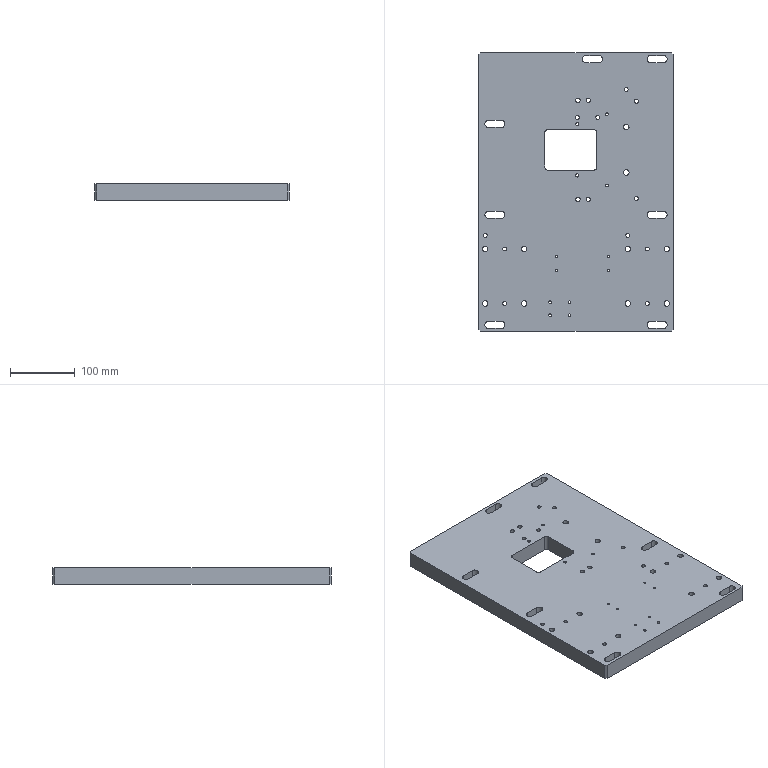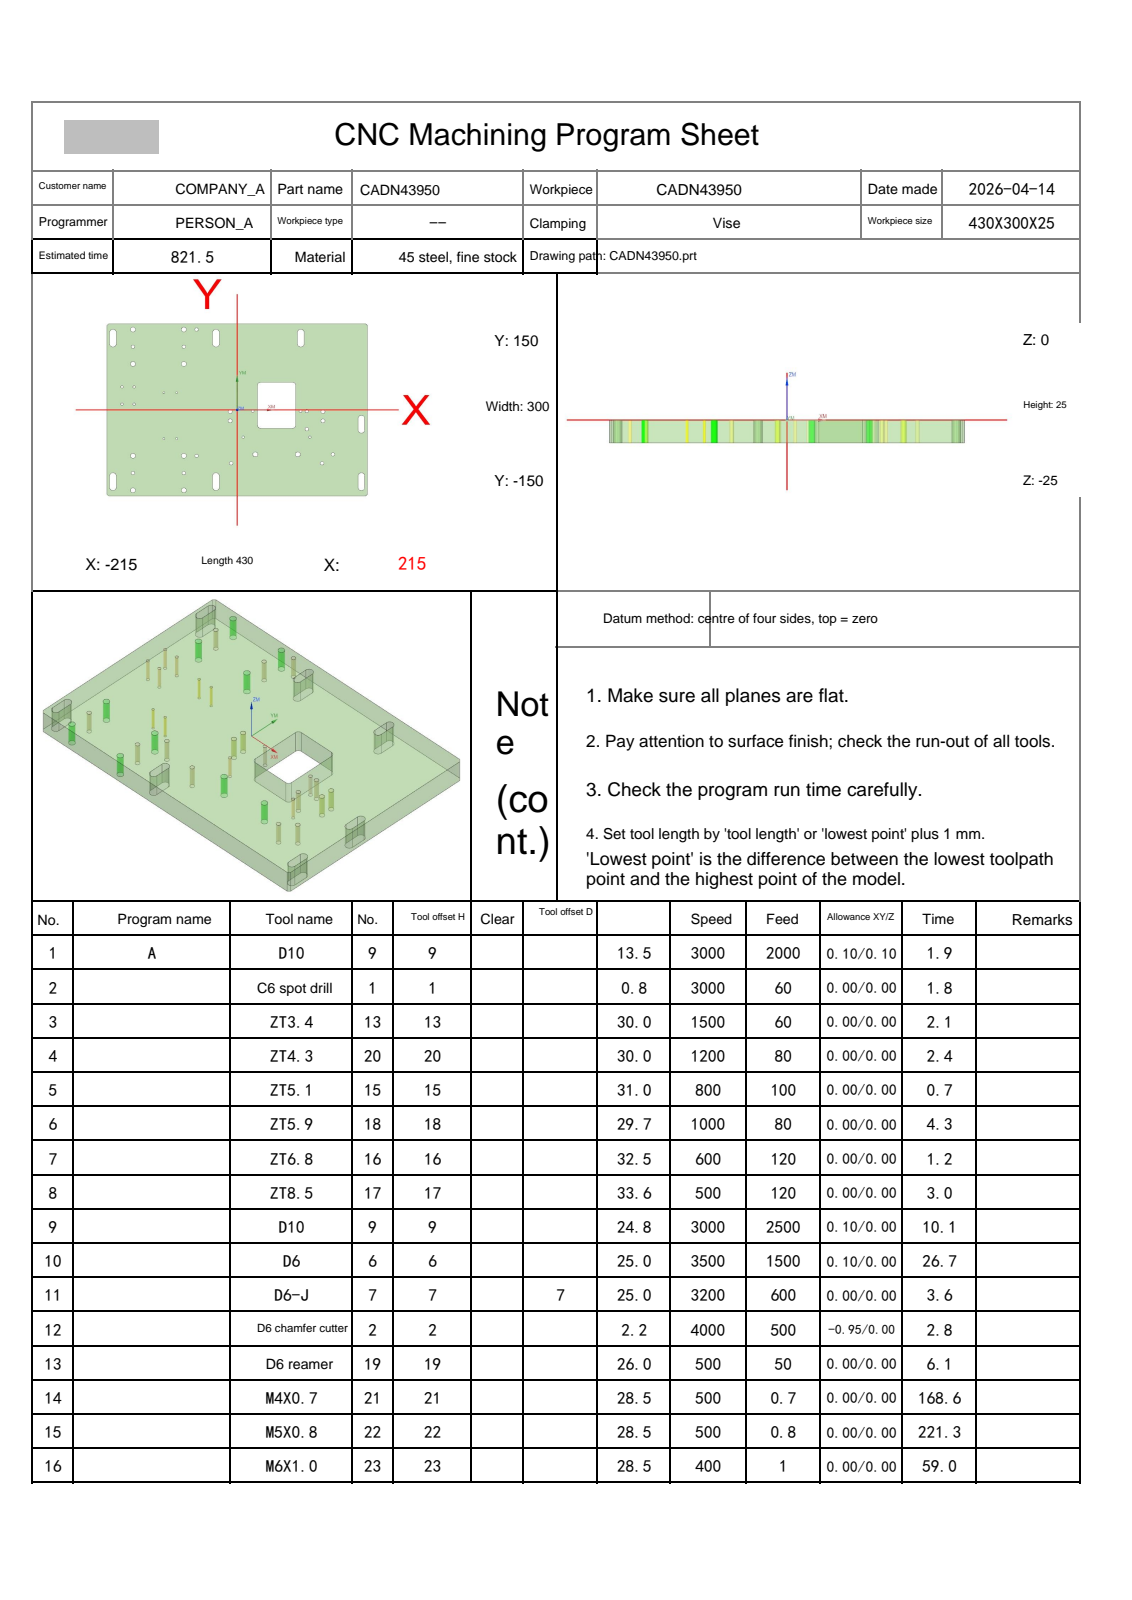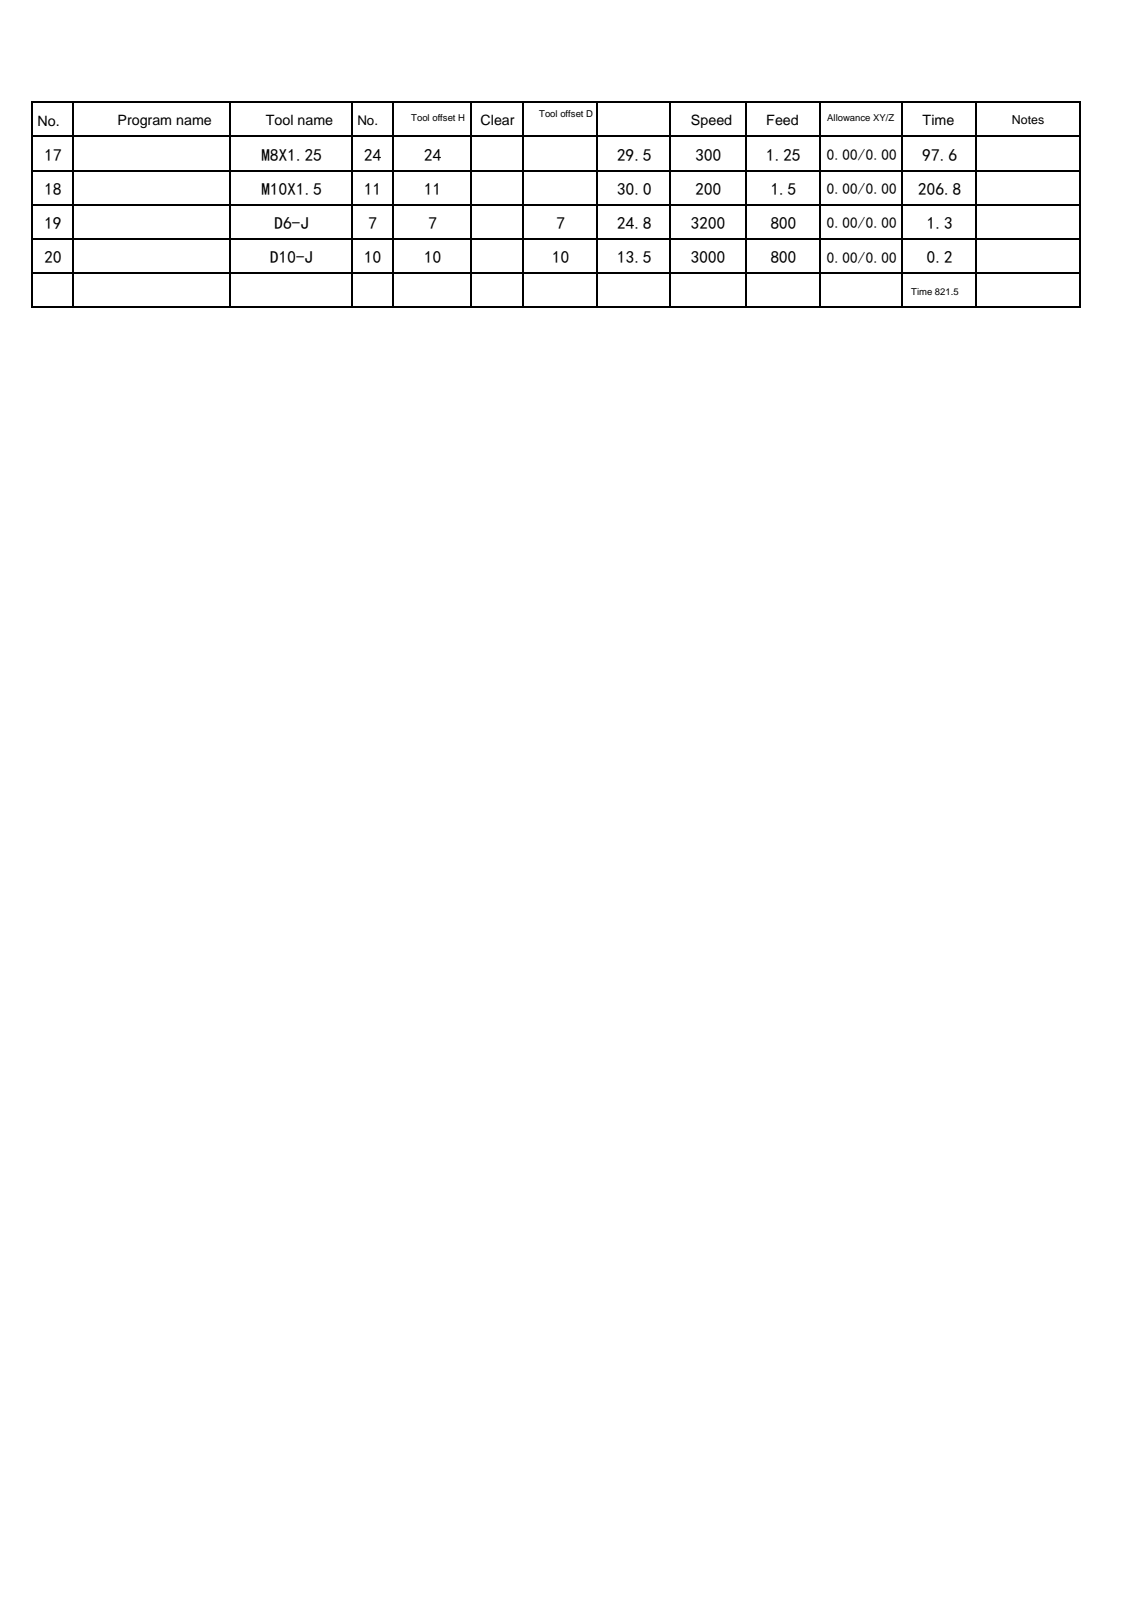NC program | NX | posted by the shop | part box 300 x 430 x 25 mm
Lines 5671 to 7024 of 7024:
N11 T07 M06
(D6-J  D=6. R=0. H=07 ce=0.00 di=0.00)
G00 G90 G54 X-207.25 Y-124.8 M03 S3200
G43 H07 Z20.
M08
Z-4.5
G01 Z-5. F600.
G41 D07
X-207.3
G03 X-207.5 Y-125. I0.0 J-.2
G01 Y-135.
G03 X-205. Y-137.5 I2.5 J0.0
X-202.5 Y-135. I0.0 J2.5
G01 Y-115.
G03 X-205. Y-112.5 I-2.5 J0.0
X-207.5 Y-115. I0.0 J-2.5
G01 Y-125.
Y-125.5
G03 X-207.3 Y-125.7 I.2 J0.0
G01 G40 X-207.25
Z-4.5
G00 Z1.
Y-124.8
Z-9.5
G01 Z-10.
G41 D07
X-207.3
G03 X-207.5 Y-125. I0.0 J-.2
G01 Y-135.
G03 X-205. Y-137.5 I2.5 J0.0
X-202.5 Y-135. I0.0 J2.5
G01 Y-115.
G03 X-205. Y-112.5 I-2.5 J0.0
X-207.5 Y-115. I0.0 J-2.5
G01 Y-125.
Y-125.5
G03 X-207.3 Y-125.7 I.2 J0.0
G01 G40 X-207.25
Z-9.5
G00 Z-4.
Y-124.8
Z-14.5
G01 Z-15.
G41 D07
X-207.3
G03 X-207.5 Y-125. I0.0 J-.2
G01 Y-135.
G03 X-205. Y-137.5 I2.5 J0.0
X-202.5 Y-135. I0.0 J2.5
G01 Y-115.
G03 X-205. Y-112.5 I-2.5 J0.0
X-207.5 Y-115. I0.0 J-2.5
G01 Y-125.
Y-125.5
G03 X-207.3 Y-125.7 I.2 J0.0
G01 G40 X-207.25
Z-14.5
G00 Z-9.
Y-124.8
Z-19.5
G01 Z-20.
G41 D07
X-207.3
G03 X-207.5 Y-125. I0.0 J-.2
G01 Y-135.
G03 X-205. Y-137.5 I2.5 J0.0
X-202.5 Y-135. I0.0 J2.5
G01 Y-115.
G03 X-205. Y-112.5 I-2.5 J0.0
X-207.5 Y-115. I0.0 J-2.5
G01 Y-125.
Y-125.5
G03 X-207.3 Y-125.7 I.2 J0.0
G01 G40 X-207.25
Z-19.5
G00 Z-14.
Y-124.8
Z-24.5
G01 Z-25.
G41 D07
X-207.3
G03 X-207.5 Y-125. I0.0 J-.2
G01 Y-135.
G03 X-205. Y-137.5 I2.5 J0.0
X-202.5 Y-135. I0.0 J2.5
G01 Y-115.
G03 X-205. Y-112.5 I-2.5 J0.0
X-207.5 Y-115. I0.0 J-2.5
G01 Y-125.
Y-125.5
G03 X-207.3 Y-125.7 I.2 J0.0
G01 G40 X-207.25
Z-24.5
G00 Z20.
X-37.25 Y-124.8
Z-4.5
G01 Z-5.
G41 D07
X-37.3
G03 X-37.5 Y-125. I0.0 J-.2
G01 Y-135.
G03 X-35. Y-137.5 I2.5 J0.0
X-32.5 Y-135. I0.0 J2.5
G01 Y-115.
G03 X-35. Y-112.5 I-2.5 J0.0
X-37.5 Y-115. I0.0 J-2.5
G01 Y-125.
Y-125.5
G03 X-37.3 Y-125.7 I.2 J0.0
G01 G40 X-37.25
Z-4.5
G00 Z1.
Y-124.8
Z-9.5
G01 Z-10.
G41 D07
X-37.3
G03 X-37.5 Y-125. I0.0 J-.2
G01 Y-135.
G03 X-35. Y-137.5 I2.5 J0.0
X-32.5 Y-135. I0.0 J2.5
G01 Y-115.
G03 X-35. Y-112.5 I-2.5 J0.0
X-37.5 Y-115. I0.0 J-2.5
G01 Y-125.
Y-125.5
G03 X-37.3 Y-125.7 I.2 J0.0
G01 G40 X-37.25
Z-9.5
G00 Z-4.
Y-124.8
Z-14.5
G01 Z-15.
G41 D07
X-37.3
G03 X-37.5 Y-125. I0.0 J-.2
G01 Y-135.
G03 X-35. Y-137.5 I2.5 J0.0
X-32.5 Y-135. I0.0 J2.5
G01 Y-115.
G03 X-35. Y-112.5 I-2.5 J0.0
X-37.5 Y-115. I0.0 J-2.5
G01 Y-125.
Y-125.5
G03 X-37.3 Y-125.7 I.2 J0.0
G01 G40 X-37.25
Z-14.5
G00 Z-9.
Y-124.8
Z-19.5
G01 Z-20.
G41 D07
X-37.3
G03 X-37.5 Y-125. I0.0 J-.2
G01 Y-135.
G03 X-35. Y-137.5 I2.5 J0.0
X-32.5 Y-135. I0.0 J2.5
G01 Y-115.
G03 X-35. Y-112.5 I-2.5 J0.0
X-37.5 Y-115. I0.0 J-2.5
G01 Y-125.
Y-125.5
G03 X-37.3 Y-125.7 I.2 J0.0
G01 G40 X-37.25
Z-19.5
G00 Z-14.
Y-124.8
Z-24.5
G01 Z-25.
G41 D07
X-37.3
G03 X-37.5 Y-125. I0.0 J-.2
G01 Y-135.
G03 X-35. Y-137.5 I2.5 J0.0
X-32.5 Y-135. I0.0 J2.5
G01 Y-115.
G03 X-35. Y-112.5 I-2.5 J0.0
X-37.5 Y-115. I0.0 J-2.5
G01 Y-125.
Y-125.5
G03 X-37.3 Y-125.7 I.2 J0.0
G01 G40 X-37.25
Z-24.5
G00 Z20.
X207.25 Y-125.2
Z-4.5
G01 Z-5.
G41 D07
X207.3
G03 X207.5 Y-125. I0.0 J.2
G01 Y-115.
G03 X205. Y-112.5 I-2.5 J0.0
X202.5 Y-115. I0.0 J-2.5
G01 Y-135.
G03 X205. Y-137.5 I2.5 J0.0
X207.5 Y-135. I0.0 J2.5
G01 Y-125.
Y-124.5
G03 X207.3 Y-124.3 I-.2 J0.0
G01 G40 X207.25
Z-4.5
G00 Z1.
Y-125.2
Z-9.5
G01 Z-10.
G41 D07
X207.3
G03 X207.5 Y-125. I0.0 J.2
G01 Y-115.
G03 X205. Y-112.5 I-2.5 J0.0
X202.5 Y-115. I0.0 J-2.5
G01 Y-135.
G03 X205. Y-137.5 I2.5 J0.0
X207.5 Y-135. I0.0 J2.5
G01 Y-125.
Y-124.5
G03 X207.3 Y-124.3 I-.2 J0.0
G01 G40 X207.25
Z-9.5
G00 Z-4.
Y-125.2
Z-14.5
G01 Z-15.
G41 D07
X207.3
G03 X207.5 Y-125. I0.0 J.2
G01 Y-115.
G03 X205. Y-112.5 I-2.5 J0.0
X202.5 Y-115. I0.0 J-2.5
G01 Y-135.
G03 X205. Y-137.5 I2.5 J0.0
X207.5 Y-135. I0.0 J2.5
G01 Y-125.
Y-124.5
G03 X207.3 Y-124.3 I-.2 J0.0
G01 G40 X207.25
Z-14.5
G00 Z-9.
Y-125.2
Z-19.5
G01 Z-20.
G41 D07
X207.3
G03 X207.5 Y-125. I0.0 J.2
G01 Y-115.
G03 X205. Y-112.5 I-2.5 J0.0
X202.5 Y-115. I0.0 J-2.5
G01 Y-135.
G03 X205. Y-137.5 I2.5 J0.0
X207.5 Y-135. I0.0 J2.5
G01 Y-125.
Y-124.5
G03 X207.3 Y-124.3 I-.2 J0.0
G01 G40 X207.25
Z-19.5
G00 Z-14.
Y-125.2
Z-24.5
G01 Z-25.
G41 D07
X207.3
G03 X207.5 Y-125. I0.0 J.2
G01 Y-115.
G03 X205. Y-112.5 I-2.5 J0.0
X202.5 Y-115. I0.0 J-2.5
G01 Y-135.
G03 X205. Y-137.5 I2.5 J0.0
X207.5 Y-135. I0.0 J2.5
G01 Y-125.
Y-124.5
G03 X207.3 Y-124.3 I-.2 J0.0
G01 G40 X207.25
Z-24.5
G00 Z20.
Y-25.2
Z-4.5
G01 Z-5.
G41 D07
X207.3
G03 X207.5 Y-25. I0.0 J.2
G01 Y-15.
G03 X205. Y-12.5 I-2.5 J0.0
X202.5 Y-15. I0.0 J-2.5
G01 Y-35.
G03 X205. Y-37.5 I2.5 J0.0
X207.5 Y-35. I0.0 J2.5
G01 Y-25.
Y-24.5
G03 X207.3 Y-24.3 I-.2 J0.0
G01 G40 X207.25
Z-4.5
G00 Z1.
Y-25.2
Z-9.5
G01 Z-10.
G41 D07
X207.3
G03 X207.5 Y-25. I0.0 J.2
G01 Y-15.
G03 X205. Y-12.5 I-2.5 J0.0
X202.5 Y-15. I0.0 J-2.5
G01 Y-35.
G03 X205. Y-37.5 I2.5 J0.0
X207.5 Y-35. I0.0 J2.5
G01 Y-25.
Y-24.5
G03 X207.3 Y-24.3 I-.2 J0.0
G01 G40 X207.25
Z-9.5
G00 Z-4.
Y-25.2
Z-14.5
G01 Z-15.
G41 D07
X207.3
G03 X207.5 Y-25. I0.0 J.2
G01 Y-15.
G03 X205. Y-12.5 I-2.5 J0.0
X202.5 Y-15. I0.0 J-2.5
G01 Y-35.
G03 X205. Y-37.5 I2.5 J0.0
X207.5 Y-35. I0.0 J2.5
G01 Y-25.
Y-24.5
G03 X207.3 Y-24.3 I-.2 J0.0
G01 G40 X207.25
Z-14.5
G00 Z-9.
Y-25.2
Z-19.5
G01 Z-20.
G41 D07
X207.3
G03 X207.5 Y-25. I0.0 J.2
G01 Y-15.
G03 X205. Y-12.5 I-2.5 J0.0
X202.5 Y-15. I0.0 J-2.5
G01 Y-35.
G03 X205. Y-37.5 I2.5 J0.0
X207.5 Y-35. I0.0 J2.5
G01 Y-25.
Y-24.5
G03 X207.3 Y-24.3 I-.2 J0.0
G01 G40 X207.25
Z-19.5
G00 Z-14.
Y-25.2
Z-24.5
G01 Z-25.
G41 D07
X207.3
G03 X207.5 Y-25. I0.0 J.2
G01 Y-15.
G03 X205. Y-12.5 I-2.5 J0.0
X202.5 Y-15. I0.0 J-2.5
G01 Y-35.
G03 X205. Y-37.5 I2.5 J0.0
X207.5 Y-35. I0.0 J2.5
G01 Y-25.
Y-24.5
G03 X207.3 Y-24.3 I-.2 J0.0
G01 G40 X207.25
Z-24.5
G00 Z20.
X107.25 Y124.8
Z-4.5
G01 Z-5.
G41 D07
X107.3
G03 X107.5 Y125. I0.0 J.2
G01 Y135.
G03 X105. Y137.5 I-2.5 J0.0
X102.5 Y135. I0.0 J-2.5
G01 Y115.
G03 X105. Y112.5 I2.5 J0.0
X107.5 Y115. I0.0 J2.5
G01 Y125.
Y125.5
G03 X107.3 Y125.7 I-.2 J0.0
G01 G40 X107.25
Z-4.5
G00 Z1.
Y124.8
Z-9.5
G01 Z-10.
G41 D07
X107.3
G03 X107.5 Y125. I0.0 J.2
G01 Y135.
G03 X105. Y137.5 I-2.5 J0.0
X102.5 Y135. I0.0 J-2.5
G01 Y115.
G03 X105. Y112.5 I2.5 J0.0
X107.5 Y115. I0.0 J2.5
G01 Y125.
Y125.5
G03 X107.3 Y125.7 I-.2 J0.0
G01 G40 X107.25
Z-9.5
G00 Z-4.
Y124.8
Z-14.5
G01 Z-15.
G41 D07
X107.3
G03 X107.5 Y125. I0.0 J.2
G01 Y135.
G03 X105. Y137.5 I-2.5 J0.0
X102.5 Y135. I0.0 J-2.5
G01 Y115.
G03 X105. Y112.5 I2.5 J0.0
X107.5 Y115. I0.0 J2.5
G01 Y125.
Y125.5
G03 X107.3 Y125.7 I-.2 J0.0
G01 G40 X107.25
Z-14.5
G00 Z-9.
Y124.8
Z-19.5
G01 Z-20.
G41 D07
X107.3
G03 X107.5 Y125. I0.0 J.2
G01 Y135.
G03 X105. Y137.5 I-2.5 J0.0
X102.5 Y135. I0.0 J-2.5
G01 Y115.
G03 X105. Y112.5 I2.5 J0.0
X107.5 Y115. I0.0 J2.5
G01 Y125.
Y125.5
G03 X107.3 Y125.7 I-.2 J0.0
G01 G40 X107.25
Z-19.5
G00 Z-14.
Y124.8
Z-24.5
G01 Z-25.
G41 D07
X107.3
G03 X107.5 Y125. I0.0 J.2
G01 Y135.
G03 X105. Y137.5 I-2.5 J0.0
X102.5 Y135. I0.0 J-2.5
G01 Y115.
G03 X105. Y112.5 I2.5 J0.0
X107.5 Y115. I0.0 J2.5
G01 Y125.
Y125.5
G03 X107.3 Y125.7 I-.2 J0.0
G01 G40 X107.25
Z-24.5
G00 Z20.
X-32.75 Y124.8
Z-4.5
G01 Z-5.
G41 D07
X-32.7
G03 X-32.5 Y125. I0.0 J.2
G01 Y135.
G03 X-35. Y137.5 I-2.5 J0.0
X-37.5 Y135. I0.0 J-2.5
G01 Y115.
G03 X-35. Y112.5 I2.5 J0.0
X-32.5 Y115. I0.0 J2.5
G01 Y125.
Y125.5
G03 X-32.7 Y125.7 I-.2 J0.0
G01 G40 X-32.75
Z-4.5
G00 Z1.
Y124.8
Z-9.5
G01 Z-10.
G41 D07
X-32.7
G03 X-32.5 Y125. I0.0 J.2
G01 Y135.
G03 X-35. Y137.5 I-2.5 J0.0
X-37.5 Y135. I0.0 J-2.5
G01 Y115.
G03 X-35. Y112.5 I2.5 J0.0
X-32.5 Y115. I0.0 J2.5
G01 Y125.
Y125.5
G03 X-32.7 Y125.7 I-.2 J0.0
G01 G40 X-32.75
Z-9.5
G00 Z-4.
Y124.8
Z-14.5
G01 Z-15.
G41 D07
X-32.7
G03 X-32.5 Y125. I0.0 J.2
G01 Y135.
G03 X-35. Y137.5 I-2.5 J0.0
X-37.5 Y135. I0.0 J-2.5
G01 Y115.
G03 X-35. Y112.5 I2.5 J0.0
X-32.5 Y115. I0.0 J2.5
G01 Y125.
Y125.5
G03 X-32.7 Y125.7 I-.2 J0.0
G01 G40 X-32.75
Z-14.5
G00 Z-9.
Y124.8
Z-19.5
G01 Z-20.
G41 D07
X-32.7
G03 X-32.5 Y125. I0.0 J.2
G01 Y135.
G03 X-35. Y137.5 I-2.5 J0.0
X-37.5 Y135. I0.0 J-2.5
G01 Y115.
G03 X-35. Y112.5 I2.5 J0.0
X-32.5 Y115. I0.0 J2.5
G01 Y125.
Y125.5
G03 X-32.7 Y125.7 I-.2 J0.0
G01 G40 X-32.75
Z-19.5
G00 Z-14.
Y124.8
Z-24.5
G01 Z-25.
G41 D07
X-32.7
G03 X-32.5 Y125. I0.0 J.2
G01 Y135.
G03 X-35. Y137.5 I-2.5 J0.0
X-37.5 Y135. I0.0 J-2.5
G01 Y115.
G03 X-35. Y112.5 I2.5 J0.0
X-32.5 Y115. I0.0 J2.5
G01 Y125.
Y125.5
G03 X-32.7 Y125.7 I-.2 J0.0
G01 G40 X-32.75
Z-24.5
G00 Z20.
X-207.25 Y125.2
Z-4.5
G01 Z-5.
G41 D07
X-207.3
G03 X-207.5 Y125. I0.0 J-.2
G01 Y115.
G03 X-205. Y112.5 I2.5 J0.0
X-202.5 Y115. I0.0 J2.5
G01 Y135.
G03 X-205. Y137.5 I-2.5 J0.0
X-207.5 Y135. I0.0 J-2.5
G01 Y125.
Y124.5
G03 X-207.3 Y124.3 I.2 J0.0
G01 G40 X-207.25
Z-4.5
G00 Z1.
Y125.2
Z-9.5
G01 Z-10.
G41 D07
X-207.3
G03 X-207.5 Y125. I0.0 J-.2
G01 Y115.
G03 X-205. Y112.5 I2.5 J0.0
X-202.5 Y115. I0.0 J2.5
G01 Y135.
G03 X-205. Y137.5 I-2.5 J0.0
X-207.5 Y135. I0.0 J-2.5
G01 Y125.
Y124.5
G03 X-207.3 Y124.3 I.2 J0.0
G01 G40 X-207.25
Z-9.5
G00 Z-4.
Y125.2
Z-14.5
G01 Z-15.
G41 D07
X-207.3
G03 X-207.5 Y125. I0.0 J-.2
G01 Y115.
G03 X-205. Y112.5 I2.5 J0.0
X-202.5 Y115. I0.0 J2.5
G01 Y135.
G03 X-205. Y137.5 I-2.5 J0.0
X-207.5 Y135. I0.0 J-2.5
G01 Y125.
Y124.5
G03 X-207.3 Y124.3 I.2 J0.0
G01 G40 X-207.25
Z-14.5
G00 Z-9.
Y125.2
Z-19.5
G01 Z-20.
G41 D07
X-207.3
G03 X-207.5 Y125. I0.0 J-.2
G01 Y115.
G03 X-205. Y112.5 I2.5 J0.0
X-202.5 Y115. I0.0 J2.5
G01 Y135.
G03 X-205. Y137.5 I-2.5 J0.0
X-207.5 Y135. I0.0 J-2.5
G01 Y125.
Y124.5
G03 X-207.3 Y124.3 I.2 J0.0
G01 G40 X-207.25
Z-19.5
G00 Z-14.
Y125.2
Z-24.5
G01 Z-25.
G41 D07
X-207.3
G03 X-207.5 Y125. I0.0 J-.2
G01 Y115.
G03 X-205. Y112.5 I2.5 J0.0
X-202.5 Y115. I0.0 J2.5
G01 Y135.
G03 X-205. Y137.5 I-2.5 J0.0
X-207.5 Y135. I0.0 J-2.5
G01 Y125.
Y124.5
G03 X-207.3 Y124.3 I.2 J0.0
G01 G40 X-207.25
Z-24.5
G00 Z20.
G91 G28 Z0.0
M05
M09
G91 G28 Z0.0
M01
N12 T02 M06
(D6 chamfer cutter D=6. R=0. H=02 ce=0.00 di=0.00)
G00 G90 G54 X-121. Y-50. M03 S4000
G43 H02 Z20.
M08
G98 G81 X-121. Y-50. Z-2.2 R3. F80.
X-100.
Y30.
X-121.
G80
G00 Z20.
G00 G90 X119.306 Y-47.593 M03 S4000
Z20.
Z-.5
G01 Z-1. F200.
X118.5 Y-47.7
G03 X120. Y-49.2 I1.5 J0.0
X121.7 Y-47.5 I0.0 J1.7
X120. Y-45.8 I-1.7 J0.0
X118.3 Y-47.5 I0.0 J-1.7
X120. Y-49.2 I1.7 J0.0
X121.5 Y-47.7 I0.0 J1.5
G01 X120.694 Y-47.593
Z-.5
G00 Z20.
X9.306
Z-.5
G01 Z-1.
X8.5 Y-47.7
G03 X10. Y-49.2 I1.5 J0.0
X11.7 Y-47.5 I0.0 J1.7
X10. Y-45.8 I-1.7 J0.0
X8.3 Y-47.5 I0.0 J-1.7
X10. Y-49.2 I1.7 J0.0
X11.5 Y-47.7 I0.0 J1.5
G01 X10.694 Y-47.593
Z-.5
G00 Z20.
X-170.694 Y9.907
Z-.5
G01 Z-1.
X-171.5 Y9.8
G03 X-170. Y8.3 I1.5 J0.0
X-168.3 Y10. I0.0 J1.7
X-170. Y11.7 I-1.7 J0.0
X-171.7 Y10. I0.0 J-1.7
X-170. Y8.3 I1.7 J0.0
X-168.5 Y9.8 I0.0 J1.5
G01 X-169.306 Y9.907
Z-.5
G00 Z20.
X-190.694
Z-.5
G01 Z-1.
X-191.5 Y9.8
G03 X-190. Y8.3 I1.5 J0.0
X-188.3 Y10. I0.0 J1.7
X-190. Y11.7 I-1.7 J0.0
X-191.7 Y10. I0.0 J-1.7
X-190. Y8.3 I1.7 J0.0
X-188.5 Y9.8 I0.0 J1.5
G01 X-189.306 Y9.907
Z-.5
G00 Z20.
X-190.694 Y39.907
Z-.5
G01 Z-1.
X-191.5 Y39.8
G03 X-190. Y38.3 I1.5 J0.0
X-188.3 Y40. I0.0 J1.7
X-190. Y41.7 I-1.7 J0.0
X-191.7 Y40. I0.0 J-1.7
X-190. Y38.3 I1.7 J0.0
X-188.5 Y39.8 I0.0 J1.5
G01 X-189.306 Y39.907
Z-.5
G00 Z20.
X-170.694
Z-.5
G01 Z-1.
X-171.5 Y39.8
G03 X-170. Y38.3 I1.5 J0.0
X-168.3 Y40. I0.0 J1.7
X-170. Y41.7 I-1.7 J0.0
X-171.7 Y40. I0.0 J-1.7
X-170. Y38.3 I1.7 J0.0
X-168.5 Y39.8 I0.0 J1.5
G01 X-169.306 Y39.907
Z-.5
G00 Z20.
G00 G90 X24.479 Y-2.409 M03 S4000
Z20.
Z-.6
G01 Z-1.1 F300.
X24. Y-2.6
G03 X25.5 Y-4.1 I1.5 J0.0
X27.6 Y-2. I0.0 J2.1
X25.5 Y.1 I-2.1 J0.0
X23.4 Y-2. I0.0 J-2.1
X25.5 Y-4.1 I2.1 J0.0
X27. Y-2.6 I0.0 J1.5
G01 X26.521 Y-2.409
Z-.6
G00 Z20.
X103.479
Z-.6
G01 Z-1.1
X103. Y-2.6
G03 X104.5 Y-4.1 I1.5 J0.0
X106.6 Y-2. I0.0 J2.1
X104.5 Y.1 I-2.1 J0.0
X102.4 Y-2. I0.0 J-2.1
X104.5 Y-4.1 I2.1 J0.0
X106. Y-2.6 I0.0 J1.5
G01 X105.521 Y-2.409
Z-.6
G00 Z20.
G00 G90 X113.853 Y-2.612 M03 S4000
Z20.
Z-.5
G01 Z-1. F400.
X113.5 Y-2.8
G03 X115. Y-4.3 I1.5 J0.0
X117.3 Y-2. I0.0 J2.3
X115. Y.3 I-2.3 J0.0
X112.7 Y-2. I0.0 J-2.3
X115. Y-4.3 I2.3 J0.0
X116.5 Y-2.8 I0.0 J1.5
G01 X116.147 Y-2.612
Z-.5
G00 Z20.
X113.853 Y-34.112
Z-.5
G01 Z-1.
X113.5 Y-34.3
G03 X115. Y-35.8 I1.5 J0.0
X117.3 Y-33.5 I0.0 J2.3
X115. Y-31.2 I-2.3 J0.0
X112.7 Y-33.5 I0.0 J-2.3
X115. Y-35.8 I2.3 J0.0
X116.5 Y-34.3 I0.0 J1.5
G01 X116.147 Y-34.112
Z-.5
G00 Z20.
X156.853 Y-78.112
Z-.5
G01 Z-1.
X156.5 Y-78.3
G03 X158. Y-79.8 I1.5 J0.0
X160.3 Y-77.5 I0.0 J2.3
X158. Y-75.2 I-2.3 J0.0
X155.7 Y-77.5 I0.0 J-2.3
X158. Y-79.8 I2.3 J0.0
X159.5 Y-78.3 I0.0 J1.5
G01 X159.147 Y-78.112
Z-.5
G00 Z20.
X138.853 Y-93.612
Z-.5
G01 Z-1.
X138.5 Y-93.8
G03 X140. Y-95.3 I1.5 J0.0
X142.3 Y-93. I0.0 J2.3
X140. Y-90.7 I-2.3 J0.0
X137.7 Y-93. I0.0 J-2.3
X140. Y-95.3 I2.3 J0.0
X141.5 Y-93.8 I0.0 J1.5
G01 X141.147 Y-93.612
Z-.5
G00 Z20.
X-11.147
Z-.5
G01 Z-1.
X-11.5 Y-93.8
G03 X-10. Y-95.3 I1.5 J0.0
X-7.7 Y-93. I0.0 J2.3
X-10. Y-90.7 I-2.3 J0.0
X-12.3 Y-93. I0.0 J-2.3
X-10. Y-95.3 I2.3 J0.0
X-8.5 Y-93.8 I0.0 J1.5
G01 X-8.853 Y-93.612
Z-.5
G00 Z20.
X-68.147 Y-80.612
Z-.5
G01 Z-1.
X-68.5 Y-80.8
G03 X-67. Y-82.3 I1.5 J0.0
X-64.7 Y-80. I0.0 J2.3
X-67. Y-77.7 I-2.3 J0.0
X-69.3 Y-80. I0.0 J-2.3
X-67. Y-82.3 I2.3 J0.0
X-65.5 Y-80.8 I0.0 J1.5
G01 X-65.853 Y-80.612
Z-.5
G00 Z20.
X-89.147 Y-110.612
Z-.5
G01 Z-1.
X-89.5 Y-110.8
G03 X-88. Y-112.3 I1.5 J0.0
X-85.7 Y-110. I0.0 J2.3
X-88. Y-107.7 I-2.3 J0.0
X-90.3 Y-110. I0.0 J-2.3
X-88. Y-112.3 I2.3 J0.0
X-86.5 Y-110.8 I0.0 J1.5
G01 X-86.853 Y-110.612
Z-.5
G00 Z20.
X-173.147
Z-.5
G01 Z-1.
X-173.5 Y-110.8
G03 X-172. Y-112.3 I1.5 J0.0
X-169.7 Y-110. I0.0 J2.3
X-172. Y-107.7 I-2.3 J0.0
X-174.3 Y-110. I0.0 J-2.3
X-172. Y-112.3 I2.3 J0.0
X-170.5 Y-110.8 I0.0 J1.5
G01 X-170.853 Y-110.612
Z-.5
G00 Z20.
X-173.147 Y109.388
Z-.5
G01 Z-1.
X-173.5 Y109.2
G03 X-172. Y107.7 I1.5 J0.0
X-169.7 Y110. I0.0 J2.3
X-172. Y112.3 I-2.3 J0.0
X-174.3 Y110. I0.0 J-2.3
X-172. Y107.7 I2.3 J0.0
X-170.5 Y109.2 I0.0 J1.5
G01 X-170.853 Y109.388
Z-.5
G00 Z20.
X-89.147
Z-.5
G01 Z-1.
X-89.5 Y109.2
G03 X-88. Y107.7 I1.5 J0.0
X-85.7 Y110. I0.0 J2.3
X-88. Y112.3 I-2.3 J0.0
X-90.3 Y110. I0.0 J-2.3
X-88. Y107.7 I2.3 J0.0
X-86.5 Y109.2 I0.0 J1.5
G01 X-86.853 Y109.388
Z-.5
G00 Z20.
X-68.147 Y139.388
Z-.5
G01 Z-1.
X-68.5 Y139.2
G03 X-67. Y137.7 I1.5 J0.0
X-64.7 Y140. I0.0 J2.3
X-67. Y142.3 I-2.3 J0.0
X-69.3 Y140. I0.0 J-2.3
X-67. Y137.7 I2.3 J0.0
X-65.5 Y139.2 I0.0 J1.5
G01 X-65.853 Y139.388
Z-.5
G00 Z20.
G00 G90 X140. Y-3.8 M03 S4000
Z20.
Z-1.
G01 Z-1.5 F500.
Y-4.2
G03 X141.5 Y-5.7 I1.5 J0.0
X144.2 Y-3. I0.0 J2.7
X141.5 Y-.3 I-2.7 J0.0
X138.8 Y-3. I0.0 J-2.7
X141.5 Y-5.7 I2.7 J0.0
X143. Y-4.2 I0.0 J1.5
G01 Y-3.8
Z-1.
G00 Z20.
X140. Y-19.8
Z-1.
G01 Z-1.5
Y-20.2
G03 X141.5 Y-21.7 I1.5 J0.0
X144.2 Y-19. I0.0 J2.7
X141.5 Y-16.3 I-2.7 J0.0
X138.8 Y-19. I0.0 J-2.7
X141.5 Y-21.7 I2.7 J0.0
X143. Y-20.2 I0.0 J1.5
G01 Y-19.8
Z-1.
G00 Z20.
X-13.
Z-1.
G01 Z-1.5
Y-20.2
G03 X-11.5 Y-21.7 I1.5 J0.0
X-8.8 Y-19. I0.0 J2.7
X-11.5 Y-16.3 I-2.7 J0.0
X-14.2 Y-19. I0.0 J-2.7
X-11.5 Y-21.7 I2.7 J0.0
X-10. Y-20.2 I0.0 J1.5
G01 Y-19.8
Z-1.
G00 Z20.
X-13. Y-3.8
Z-1.
G01 Z-1.5
Y-4.2
G03 X-11.5 Y-5.7 I1.5 J0.0
X-8.8 Y-3. I0.0 J2.7
X-11.5 Y-.3 I-2.7 J0.0
X-14.2 Y-3. I0.0 J-2.7
X-11.5 Y-5.7 I2.7 J0.0
X-10. Y-4.2 I0.0 J1.5
G01 Y-3.8
Z-1.
G00 Z20.
G00 G90 X97.371 Y-78.114 M03 S4000
Z20.
Z-1.
G01 Z-1.5 F500.
X97. Y-78.2
G03 X100. Y-81.2 I3. J0.0
X103.7 Y-77.5 I0.0 J3.7
X100. Y-73.8 I-3.7 J0.0
X96.3 Y-77.5 I0.0 J-3.7
X100. Y-81.2 I3.7 J0.0
X103. Y-78.2 I0.0 J3.
G01 X102.629 Y-78.114
Z-1.
G00 Z20.
X27.371
Z-1.
G01 Z-1.5
X27. Y-78.2
G03 X30. Y-81.2 I3. J0.0
X33.7 Y-77.5 I0.0 J3.7
X30. Y-73.8 I-3.7 J0.0
X26.3 Y-77.5 I0.0 J-3.7
X30. Y-81.2 I3.7 J0.0
X33. Y-78.2 I0.0 J3.
G01 X32.629 Y-78.114
Z-1.
G00 Z20.
X-90.629 Y-80.614
Z-1.
G01 Z-1.5
X-91. Y-80.7
G03 X-88. Y-83.7 I3. J0.0
X-84.3 Y-80. I0.0 J3.7
X-88. Y-76.3 I-3.7 J0.0
X-91.7 Y-80. I0.0 J-3.7
X-88. Y-83.7 I3.7 J0.0
X-85. Y-80.7 I0.0 J3.
G01 X-85.371 Y-80.614
Z-1.
G00 Z20.
X-90.629 Y-140.614
Z-1.
G01 Z-1.5
X-91. Y-140.7
G03 X-88. Y-143.7 I3. J0.0
X-84.3 Y-140. I0.0 J3.7
X-88. Y-136.3 I-3.7 J0.0
X-91.7 Y-140. I0.0 J-3.7
X-88. Y-143.7 I3.7 J0.0
X-85. Y-140.7 I0.0 J3.
G01 X-85.371 Y-140.614
Z-1.
G00 Z20.
X-174.629
Z-1.
G01 Z-1.5
X-175. Y-140.7
G03 X-172. Y-143.7 I3. J0.0
X-168.3 Y-140. I0.0 J3.7
X-172. Y-136.3 I-3.7 J0.0
X-175.7 Y-140. I0.0 J-3.7
X-172. Y-143.7 I3.7 J0.0
X-169. Y-140.7 I0.0 J3.
G01 X-169.371 Y-140.614
Z-1.
G00 Z20.
X-174.629 Y-80.614
Z-1.
G01 Z-1.5
X-175. Y-80.7
G03 X-172. Y-83.7 I3. J0.0
X-168.3 Y-80. I0.0 J3.7
X-172. Y-76.3 I-3.7 J0.0
X-175.7 Y-80. I0.0 J-3.7
X-172. Y-83.7 I3.7 J0.0
X-169. Y-80.7 I0.0 J3.
G01 X-169.371 Y-80.614
Z-1.
G00 Z20.
X-174.629 Y79.386
Z-1.
G01 Z-1.5
X-175. Y79.3
G03 X-172. Y76.3 I3. J0.0
X-168.3 Y80. I0.0 J3.7
X-172. Y83.7 I-3.7 J0.0
X-175.7 Y80. I0.0 J-3.7
X-172. Y76.3 I3.7 J0.0
X-169. Y79.3 I0.0 J3.
G01 X-169.371 Y79.386
Z-1.
G00 Z20.
X-174.629 Y139.386
Z-1.
G01 Z-1.5
X-175. Y139.3
G03 X-172. Y136.3 I3. J0.0
X-168.3 Y140. I0.0 J3.7
X-172. Y143.7 I-3.7 J0.0
X-175.7 Y140. I0.0 J-3.7
X-172. Y136.3 I3.7 J0.0
X-169. Y139.3 I0.0 J3.
G01 X-169.371 Y139.386
Z-1.
G00 Z20.
X-90.629
Z-1.
G01 Z-1.5
X-91. Y139.3
G03 X-88. Y136.3 I3. J0.0
X-84.3 Y140. I0.0 J3.7
X-88. Y143.7 I-3.7 J0.0
X-91.7 Y140. I0.0 J-3.7
X-88. Y136.3 I3.7 J0.0
X-85. Y139.3 I0.0 J3.
G01 X-85.371 Y139.386
Z-1.
G00 Z20.
X-90.629 Y79.386
Z-1.
G01 Z-1.5
X-91. Y79.3
G03 X-88. Y76.3 I3. J0.0
X-84.3 Y80. I0.0 J3.7
X-88. Y83.7 I-3.7 J0.0
X-91.7 Y80. I0.0 J-3.7
X-88. Y76.3 I3.7 J0.0
X-85. Y79.3 I0.0 J3.
G01 X-85.371 Y79.386
Z-1.
G00 Z20.
G91 G28 Z0.0
M05
M09
G91 G28 Z0.0
M01
N13 T19 M06
(D6 reamer D=6. DR_a=180 H=19)
G00 G90 G54 X-67. Y140. M03 S500
G43 H19 Z20.
M08
G98 G81 X-67. Y140. Z-26. R1. F50.
X-88. Y110.
X-172.
Y-110.
X-88.
X-67. Y-80.
X-10. Y-93.
X140.
X158. Y-77.5
X115. Y-33.5
Y-2.
G80
G00 Z20.
G91 G28 Z0.0
M05
M09
G91 G28 Z0.0
M01
N14 T21 M06
(M4X0.7 D=3.3 DR_a=180 H=21)
G00 G90 G54 X-121. Y-50. M03 S500
G43 H21 Z20.
M08
G95
G98 G84 X-121. Y-50. Z-28.5 R1. F.7 Q1.
X-100.
Y30.
X-121.
G80
G94
G00 Z20.
G91 G28 Z0.0
M05
M09
G91 G28 Z0.0
M01
N15 T22 M06
(M5X0.8 D=4.2 DR_a=180 H=22)
G00 G90 G54 X-170. Y40. M03 S500
G43 H22 Z20.
M08
G95
G98 G84 X-170. Y40. Z-28.5 R1. F.8 Q2.
X-190.
Y10.
X-170.
X10. Y-47.5
X120.
G80
G94
G00 Z20.
G91 G28 Z0.0
M05
M09
G91 G28 Z0.0
M01
N16 T23 M06
(M6X1.0 D=5. DR_a=180 H=23)
G00 G90 G54 X25.5 Y-2. M03 S400
G43 H23 Z20.
M08
G95
G98 G84 X25.5 Y-2. Z-28.5 R1. F1. Q2.
X104.5
G80
G94
G00 Z20.
G91 G28 Z0.0
M05
M09
G91 G28 Z0.0
M01
N17 T24 M06
(M8X1.25 D=6.8 DR_a=180 H=24)
G00 G90 G54 X141.5 Y-3. M03 S300
G43 H24 Z20.
M08
G95
G98 G84 X141.5 Y-3. Z-29.5 R1. F1.25 Q3.
Y-19.
X-11.5
Y-3.
G80
G94
G00 Z20.
G91 G28 Z0.0
M05
M09
G91 G28 Z0.0
M01
N18 T11 M06
(M10X1.5 D=8.5 DR_a=180 H=11)
G00 G90 G54 X-88. Y80. M03 S200
G43 H11 Z20.
M08
G95
G98 G84 X-88. Y80. Z-30. R1. F1.5 Q2.
Y140.
X-172.
Y80.
Y-80.
Y-140.
X-88.
Y-80.
X30. Y-77.5
X100.
G80
G94
G00 Z20.
G91 G28 Z0.0
M05
M09
G91 G28 Z0.0
M01
N19 T07 M06
(D6-J  D=6. R=0. H=07 ce=0.00 di=0.00)
G00 G90 G54 X91.3 Y-28. M03 S3200
G43 H07 Z20.
M08
Z-7.667
G01 Z-8.167 F720.
G41 D07
X92.5
G03 X93.5 Y-27. I0.0 J1.
G01 Y43. F800.
G03 X91.5 Y45. I-2. J0.0
G01 X38.5
G03 X36.5 Y43. I0.0 J-2.
G01 Y-27.
G03 X38.5 Y-29. I2. J0.0
G01 X91.5
G03 X93.5 Y-27. I0.0 J2.
G01 Y-26.5
G03 X92.5 Y-25.5 I-1. J0.0
G01 G40 X92.3
Z-7.667
G00 X91.3 Y-28.
Z-15.833
G01 Z-16.333 F720.
G41 D07
X92.5
G03 X93.5 Y-27. I0.0 J1.
G01 Y43. F800.
G03 X91.5 Y45. I-2. J0.0
G01 X38.5
G03 X36.5 Y43. I0.0 J-2.
G01 Y-27.
G03 X38.5 Y-29. I2. J0.0
G01 X91.5
G03 X93.5 Y-27. I0.0 J2.
G01 Y-26.5
G03 X92.5 Y-25.5 I-1. J0.0
G01 G40 X92.3
Z-15.833
G00 X91.3 Y-28.
Z-24.
G01 Z-24.5 F720.
G41 D07
X92.5
G03 X93.5 Y-27. I0.0 J1.
G01 Y43. F800.
G03 X91.5 Y45. I-2. J0.0
G01 X38.5
G03 X36.5 Y43. I0.0 J-2.
G01 Y-27.
G03 X38.5 Y-29. I2. J0.0
G01 X91.5
G03 X93.5 Y-27. I0.0 J2.
G01 Y-26.5
G03 X92.5 Y-25.5 I-1. J0.0
G01 G40 X92.3
Z-24.
G00 Z20.
G00 G90 X92.207 Y-27.707 M03 S3200
Z20.
Z-24.3
G01 Z-24.8 F720.
G41 D07
X92.5 Y-28.
G03 X93.5 Y-27. I0.0 J1.
G01 Y43. F800.
G03 X91.5 Y45. I-2. J0.0
G01 X38.5
G03 X36.5 Y43. I0.0 J-2.
G01 Y-27.
G03 X38.5 Y-29. I2. J0.0
G01 X91.5
G03 X93.5 Y-27. I0.0 J2.
G01 Y-26.5
G03 X92.5 Y-25.5 I-1. J0.0
G01 G40 X92.4
Z-24.3
G00 Z20.
G91 G28 Z0.0
M05
M09
G91 G28 Z0.0
M01
N20 T10 M06
(D10-J  D=10. R=0. H=10 ce=0.00 di=0.00)
G00 G90 G54 X215.544 Y155.684 M03 S3000
G43 H10 Z5.
M08
Z-12.5
G01 Z-13.5 F800.
G41 D10
X215.42 Y155.527
G03 X215.096 Y154.596 I1.176 J-.931
X215.536 Y153.536 I1.5 J0.0
G01 X218.536 Y150.536
G03 X219.596 Y150.096 I1.061 J1.061
X220.527 Y150.42 I0.0 J1.5
G01 G40 X220.684 Y150.544
Z-12.5
G00 Z5.
Y-150.544
Z-12.5
G01 Z-13.5
G41 D10
X220.527 Y-150.42
G03 X219.596 Y-150.096 I-.931 J-1.176
X218.536 Y-150.536 I0.0 J-1.5
G01 X215.536 Y-153.536
G03 X215.096 Y-154.596 I1.061 J-1.061
X215.42 Y-155.527 I1.5 J0.0
G01 G40 X215.544 Y-155.684
Z-12.5
G00 Z5.
X-215.544
Z-12.5
G01 Z-13.5
G41 D10
X-215.42 Y-155.527
G03 X-215.096 Y-154.596 I-1.176 J.931
X-215.536 Y-153.536 I-1.5 J0.0
G01 X-218.536 Y-150.536
G03 X-219.596 Y-150.096 I-1.061 J-1.061
X-220.527 Y-150.42 I0.0 J-1.5
G01 G40 X-220.684 Y-150.544
Z-12.5
G00 Z5.
Y150.544
Z-12.5
G01 Z-13.5
G41 D10
X-220.527 Y150.42
G03 X-219.596 Y150.096 I.931 J1.176
X-218.536 Y150.536 I0.0 J1.5
G01 X-215.536 Y153.536
G03 X-215.096 Y154.596 I-1.061 J1.061
X-215.42 Y155.527 I-1.5 J0.0
G01 G40 X-215.544 Y155.684
Z-12.5
G00 Z5.
M05
M09
G91 G28 Z0.0
G91 G28 Y0.0
M30
%